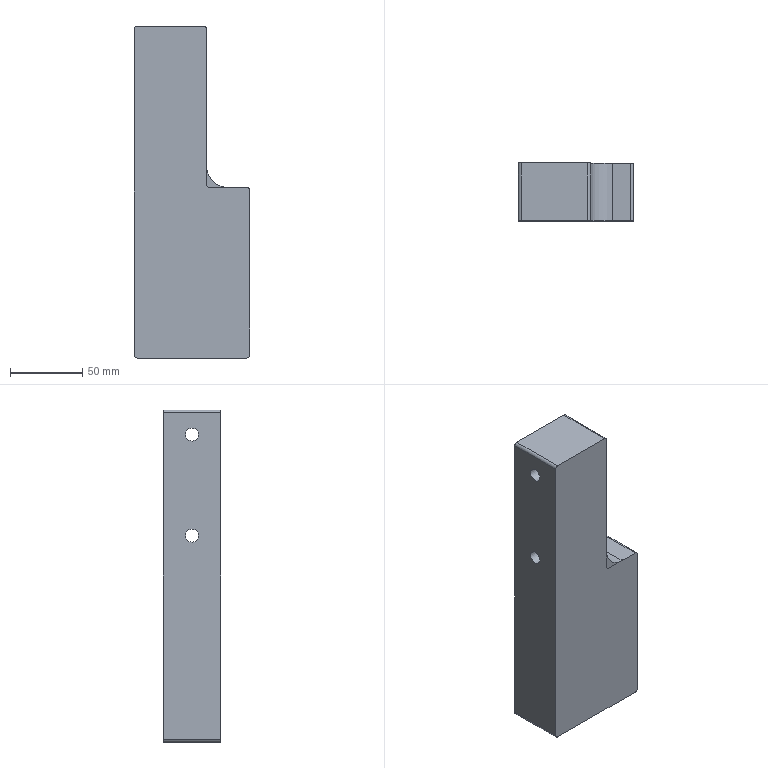NC program | NX | posted with a generic post | part box 80 x 40 x 230 mm
Lines 1 to 22 of 15398:
N10 G17 G21 G94 G90
(FLOOR_FACING_COPY_2_1 , TOOL : D40.)
N12 T18 M6
N14 G53
N16 G17 G0 G90 X-145. Y30. B0. C0. S1600 M3
N18 G43 Z50. H18
N20 Z3.1
N22 G94 G1 Z0.1 F1000.
N24 X-135.
N26 X135.
N28 Y3.
N30 X-135.
N32 Y-24.
N34 X128.205
N36 X140.77
N38 Z3.1
N40 G0 Z50.
N42 M5